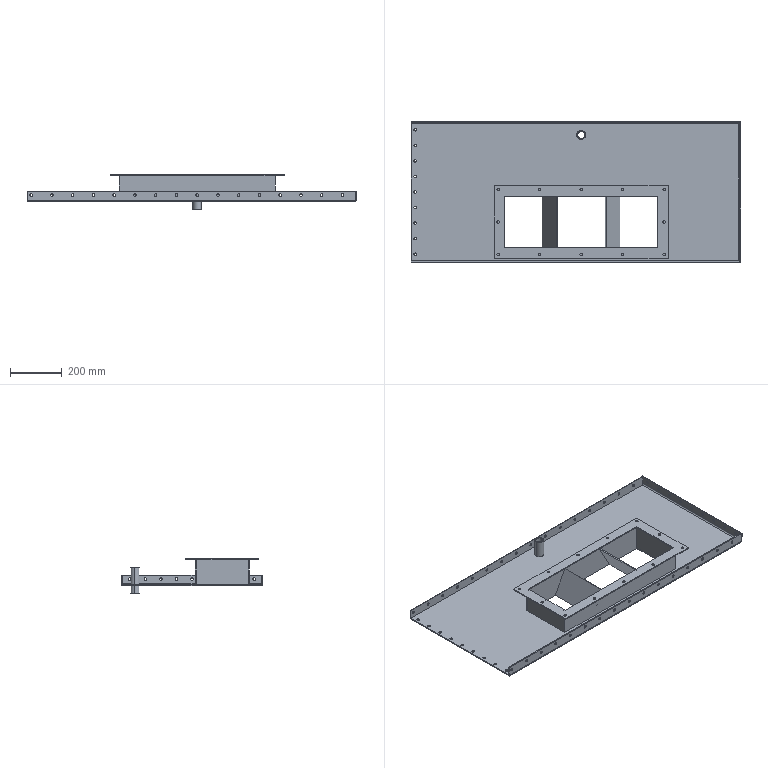Part | SolidWorks | 11 solids | 214 faces | box 1270 x 540 x 134 mm | volume 3784835 mm3 | cylinder 132 | plane 78 | cone 4 | commonest cylinder face diameters 10 x125 27 x2 33.5 x2 35 x2 18 x1